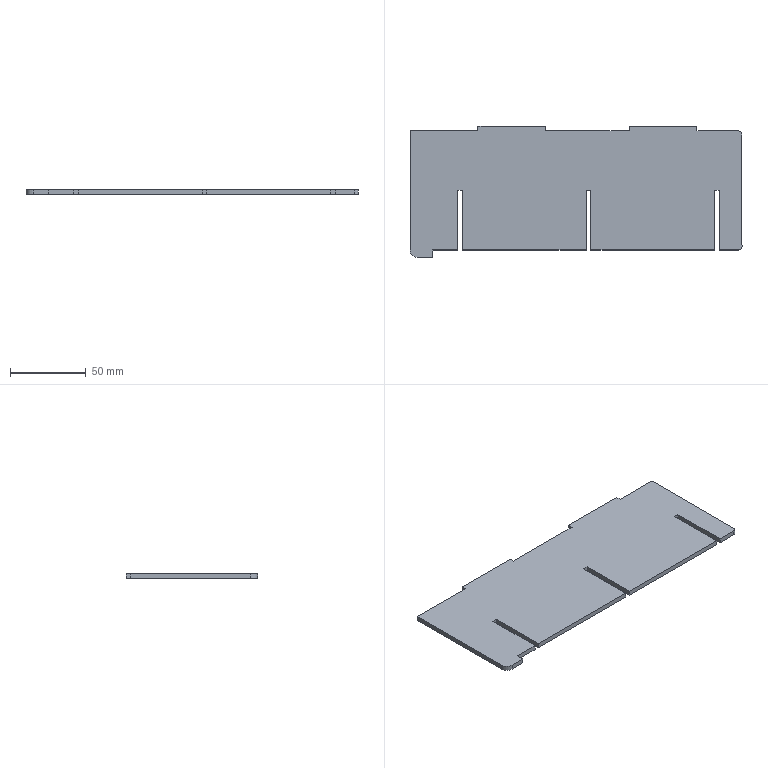Part | SolidWorks | features FlatPattern 1, SMBaseFlange 1, SheetMetal 1 | 1 solid | 31 faces | box 219.8 x 86.8 x 3.2 mm | volume 55293 mm3 | plane 28 | cylinder 3 | commonest cylinder face diameters 4 x2 10 x1
STEP:
#1=CARTESIAN_POINT('',(-115.113,-280.,0.));
#2=VERTEX_POINT('',#1);
#3=CARTESIAN_POINT('',(-98.513,-280.,0.));
#4=VERTEX_POINT('',#3);
#5=CARTESIAN_POINT('',(-98.513,-280.,0.));
#6=DIRECTION('',(1.,0.,0.));
#7=VECTOR('',#6,1000.);
#8=LINE('',#5,#7);
#9=EDGE_CURVE('',#2,#4,#8,.T.);
#10=ORIENTED_EDGE('',*,*,#9,.T.);
#11=CARTESIAN_POINT('',(-98.513,-280.,3.2));
#12=VERTEX_POINT('',#11);
#13=CARTESIAN_POINT('',(-98.513,-280.,3.2));
#14=DIRECTION('',(0.,0.,-1.));
#15=VECTOR('',#14,1000.);
#16=LINE('',#13,#15);
#17=EDGE_CURVE('',#12,#4,#16,.T.);
#18=ORIENTED_EDGE('',*,*,#17,.F.);
#19=CARTESIAN_POINT('',(-115.113,-280.,3.2));
#20=VERTEX_POINT('',#19);
#21=CARTESIAN_POINT('',(-98.513,-280.,3.2));
#22=DIRECTION('',(1.,0.,0.));
#23=VECTOR('',#22,1000.);
#24=LINE('',#21,#23);
#25=EDGE_CURVE('',#20,#12,#24,.T.);
#26=ORIENTED_EDGE('',*,*,#25,.F.);
#27=CARTESIAN_POINT('',(-115.113,-280.,3.2));
#28=DIRECTION('',(0.,0.,-1.));
#29=VECTOR('',#28,1000.);
#30=LINE('',#27,#29);
#31=EDGE_CURVE('',#20,#2,#30,.T.);
#32=ORIENTED_EDGE('',*,*,#31,.T.);
#33=EDGE_LOOP('',(#10,#18,#26,#32));
#34=FACE_OUTER_BOUND('',#33,.T.);
#35=CARTESIAN_POINT('',(-98.513,-280.,3.2));
#36=DIRECTION('',(0.,1.,0.));
#37=DIRECTION('',(-1.,0.,0.));
#38=AXIS2_PLACEMENT_3D('',#35,#36,#37);
#39=PLANE('',#38);
#40=ADVANCED_FACE('',(#34),#39,.F.);
#41=CARTESIAN_POINT('',(-98.513,-240.5,0.));
#42=VERTEX_POINT('',#41);
#43=CARTESIAN_POINT('',(-98.513,-280.,0.));
#44=DIRECTION('',(0.,1.,0.));
#45=VECTOR('',#44,1000.);
#46=LINE('',#43,#45);
#47=EDGE_CURVE('',#4,#42,#46,.T.);
#48=ORIENTED_EDGE('',*,*,#47,.T.);
#49=CARTESIAN_POINT('',(-98.513,-240.5,3.2));
#50=VERTEX_POINT('',#49);
#51=CARTESIAN_POINT('',(-98.513,-240.5,3.2));
#52=DIRECTION('',(0.,0.,-1.));
#53=VECTOR('',#52,1000.);
#54=LINE('',#51,#53);
#55=EDGE_CURVE('',#50,#42,#54,.T.);
#56=ORIENTED_EDGE('',*,*,#55,.F.);
#57=CARTESIAN_POINT('',(-98.513,-280.,3.2));
#58=DIRECTION('',(0.,1.,0.));
#59=VECTOR('',#58,1000.);
#60=LINE('',#57,#59);
#61=EDGE_CURVE('',#12,#50,#60,.T.);
#62=ORIENTED_EDGE('',*,*,#61,.F.);
#63=ORIENTED_EDGE('',*,*,#17,.T.);
#64=EDGE_LOOP('',(#48,#56,#62,#63));
#65=FACE_OUTER_BOUND('',#64,.T.);
#66=CARTESIAN_POINT('',(-98.513,-280.,3.2));
#67=DIRECTION('',(-1.,0.,0.));
#68=DIRECTION('',(0.,-1.,0.));
#69=AXIS2_PLACEMENT_3D('',#66,#67,#68);
#70=PLANE('',#69);
#71=ADVANCED_FACE('',(#65),#70,.F.);
#72=CARTESIAN_POINT('',(-95.313,-240.5,0.));
#73=VERTEX_POINT('',#72);
#74=CARTESIAN_POINT('',(-98.513,-240.5,0.));
#75=DIRECTION('',(1.,0.,0.));
#76=VECTOR('',#75,1000.);
#77=LINE('',#74,#76);
#78=EDGE_CURVE('',#42,#73,#77,.T.);
#79=ORIENTED_EDGE('',*,*,#78,.T.);
#80=CARTESIAN_POINT('',(-95.313,-240.5,3.2));
#81=VERTEX_POINT('',#80);
#82=CARTESIAN_POINT('',(-95.313,-240.5,3.2));
#83=DIRECTION('',(0.,0.,-1.));
#84=VECTOR('',#83,1000.);
#85=LINE('',#82,#84);
#86=EDGE_CURVE('',#81,#73,#85,.T.);
#87=ORIENTED_EDGE('',*,*,#86,.F.);
#88=CARTESIAN_POINT('',(-98.513,-240.5,3.2));
#89=DIRECTION('',(1.,0.,0.));
#90=VECTOR('',#89,1000.);
#91=LINE('',#88,#90);
#92=EDGE_CURVE('',#50,#81,#91,.T.);
#93=ORIENTED_EDGE('',*,*,#92,.F.);
#94=ORIENTED_EDGE('',*,*,#55,.T.);
#95=EDGE_LOOP('',(#79,#87,#93,#94));
#96=FACE_OUTER_BOUND('',#95,.T.);
#97=CARTESIAN_POINT('',(-98.513,-240.5,3.2));
#98=DIRECTION('',(0.,1.,0.));
#99=DIRECTION('',(0.,0.,1.));
#100=AXIS2_PLACEMENT_3D('',#97,#98,#99);
#101=PLANE('',#100);
#102=ADVANCED_FACE('',(#96),#101,.F.);
#103=CARTESIAN_POINT('',(-95.313,-280.,0.));
#104=VERTEX_POINT('',#103);
#105=CARTESIAN_POINT('',(-95.313,-240.5,0.));
#106=DIRECTION('',(0.,-1.,0.));
#107=VECTOR('',#106,1000.);
#108=LINE('',#105,#107);
#109=EDGE_CURVE('',#73,#104,#108,.T.);
#110=ORIENTED_EDGE('',*,*,#109,.T.);
#111=CARTESIAN_POINT('',(-95.313,-280.,3.2));
#112=VERTEX_POINT('',#111);
#113=CARTESIAN_POINT('',(-95.313,-280.,3.2));
#114=DIRECTION('',(0.,0.,-1.));
#115=VECTOR('',#114,1000.);
#116=LINE('',#113,#115);
#117=EDGE_CURVE('',#112,#104,#116,.T.);
#118=ORIENTED_EDGE('',*,*,#117,.F.);
#119=CARTESIAN_POINT('',(-95.313,-240.5,3.2));
#120=DIRECTION('',(0.,-1.,0.));
#121=VECTOR('',#120,1000.);
#122=LINE('',#119,#121);
#123=EDGE_CURVE('',#81,#112,#122,.T.);
#124=ORIENTED_EDGE('',*,*,#123,.F.);
#125=ORIENTED_EDGE('',*,*,#86,.T.);
#126=EDGE_LOOP('',(#110,#118,#124,#125));
#127=FACE_OUTER_BOUND('',#126,.T.);
#128=CARTESIAN_POINT('',(-95.313,-240.5,3.2));
#129=DIRECTION('',(1.,0.,0.));
#130=DIRECTION('',(0.,1.,0.));
#131=AXIS2_PLACEMENT_3D('',#128,#129,#130);
#132=PLANE('',#131);
#133=ADVANCED_FACE('',(#127),#132,.F.);
#134=CARTESIAN_POINT('',(-13.513,-280.,0.));
#135=VERTEX_POINT('',#134);
#136=CARTESIAN_POINT('',(-13.513,-280.,0.));
#137=DIRECTION('',(1.,0.,0.));
#138=VECTOR('',#137,1000.);
#139=LINE('',#136,#138);
#140=EDGE_CURVE('',#104,#135,#139,.T.);
#141=ORIENTED_EDGE('',*,*,#140,.T.);
#142=CARTESIAN_POINT('',(-13.513,-280.,3.2));
#143=VERTEX_POINT('',#142);
#144=CARTESIAN_POINT('',(-13.513,-280.,3.2));
#145=DIRECTION('',(0.,0.,-1.));
#146=VECTOR('',#145,1000.);
#147=LINE('',#144,#146);
#148=EDGE_CURVE('',#143,#135,#147,.T.);
#149=ORIENTED_EDGE('',*,*,#148,.F.);
#150=CARTESIAN_POINT('',(-13.513,-280.,3.2));
#151=DIRECTION('',(1.,0.,0.));
#152=VECTOR('',#151,1000.);
#153=LINE('',#150,#152);
#154=EDGE_CURVE('',#112,#143,#153,.T.);
#155=ORIENTED_EDGE('',*,*,#154,.F.);
#156=ORIENTED_EDGE('',*,*,#117,.T.);
#157=EDGE_LOOP('',(#141,#149,#155,#156));
#158=FACE_OUTER_BOUND('',#157,.T.);
#159=CARTESIAN_POINT('',(-13.513,-280.,3.2));
#160=DIRECTION('',(0.,1.,0.));
#161=DIRECTION('',(-1.,0.,0.));
#162=AXIS2_PLACEMENT_3D('',#159,#160,#161);
#163=PLANE('',#162);
#164=ADVANCED_FACE('',(#158),#163,.F.);
#165=CARTESIAN_POINT('',(-13.513,-240.5,0.));
#166=VERTEX_POINT('',#165);
#167=CARTESIAN_POINT('',(-13.513,-240.5,0.));
#168=DIRECTION('',(0.,1.,0.));
#169=VECTOR('',#168,1000.);
#170=LINE('',#167,#169);
#171=EDGE_CURVE('',#135,#166,#170,.T.);
#172=ORIENTED_EDGE('',*,*,#171,.T.);
#173=CARTESIAN_POINT('',(-13.513,-240.5,3.2));
#174=VERTEX_POINT('',#173);
#175=CARTESIAN_POINT('',(-13.513,-240.5,3.2));
#176=DIRECTION('',(0.,0.,-1.));
#177=VECTOR('',#176,1000.);
#178=LINE('',#175,#177);
#179=EDGE_CURVE('',#174,#166,#178,.T.);
#180=ORIENTED_EDGE('',*,*,#179,.F.);
#181=CARTESIAN_POINT('',(-13.513,-240.5,3.2));
#182=DIRECTION('',(0.,1.,0.));
#183=VECTOR('',#182,1000.);
#184=LINE('',#181,#183);
#185=EDGE_CURVE('',#143,#174,#184,.T.);
#186=ORIENTED_EDGE('',*,*,#185,.F.);
#187=ORIENTED_EDGE('',*,*,#148,.T.);
#188=EDGE_LOOP('',(#172,#180,#186,#187));
#189=FACE_OUTER_BOUND('',#188,.T.);
#190=CARTESIAN_POINT('',(-13.513,-240.5,3.2));
#191=DIRECTION('',(-1.,0.,0.));
#192=DIRECTION('',(0.,-1.,0.));
#193=AXIS2_PLACEMENT_3D('',#190,#191,#192);
#194=PLANE('',#193);
#195=ADVANCED_FACE('',(#189),#194,.F.);
#196=CARTESIAN_POINT('',(-10.313,-240.5,0.));
#197=VERTEX_POINT('',#196);
#198=CARTESIAN_POINT('',(-10.313,-240.5,0.));
#199=DIRECTION('',(1.,0.,0.));
#200=VECTOR('',#199,1000.);
#201=LINE('',#198,#200);
#202=EDGE_CURVE('',#166,#197,#201,.T.);
#203=ORIENTED_EDGE('',*,*,#202,.T.);
#204=CARTESIAN_POINT('',(-10.313,-240.5,3.2));
#205=VERTEX_POINT('',#204);
#206=CARTESIAN_POINT('',(-10.313,-240.5,3.2));
#207=DIRECTION('',(0.,0.,-1.));
#208=VECTOR('',#207,1000.);
#209=LINE('',#206,#208);
#210=EDGE_CURVE('',#205,#197,#209,.T.);
#211=ORIENTED_EDGE('',*,*,#210,.F.);
#212=CARTESIAN_POINT('',(-10.313,-240.5,3.2));
#213=DIRECTION('',(1.,0.,0.));
#214=VECTOR('',#213,1000.);
#215=LINE('',#212,#214);
#216=EDGE_CURVE('',#174,#205,#215,.T.);
#217=ORIENTED_EDGE('',*,*,#216,.F.);
#218=ORIENTED_EDGE('',*,*,#179,.T.);
#219=EDGE_LOOP('',(#203,#211,#217,#218));
#220=FACE_OUTER_BOUND('',#219,.T.);
#221=CARTESIAN_POINT('',(-10.313,-240.5,3.2));
#222=DIRECTION('',(0.,1.,0.));
#223=DIRECTION('',(0.,0.,1.));
#224=AXIS2_PLACEMENT_3D('',#221,#222,#223);
#225=PLANE('',#224);
#226=ADVANCED_FACE('',(#220),#225,.F.);
#227=CARTESIAN_POINT('',(-10.313,-280.,0.));
#228=VERTEX_POINT('',#227);
#229=CARTESIAN_POINT('',(-10.313,-280.,0.));
#230=DIRECTION('',(0.,-1.,0.));
#231=VECTOR('',#230,1000.);
#232=LINE('',#229,#231);
#233=EDGE_CURVE('',#197,#228,#232,.T.);
#234=ORIENTED_EDGE('',*,*,#233,.T.);
#235=CARTESIAN_POINT('',(-10.313,-280.,3.2));
#236=VERTEX_POINT('',#235);
#237=CARTESIAN_POINT('',(-10.313,-280.,3.2));
#238=DIRECTION('',(0.,0.,-1.));
#239=VECTOR('',#238,1000.);
#240=LINE('',#237,#239);
#241=EDGE_CURVE('',#236,#228,#240,.T.);
#242=ORIENTED_EDGE('',*,*,#241,.F.);
#243=CARTESIAN_POINT('',(-10.313,-280.,3.2));
#244=DIRECTION('',(0.,-1.,0.));
#245=VECTOR('',#244,1000.);
#246=LINE('',#243,#245);
#247=EDGE_CURVE('',#205,#236,#246,.T.);
#248=ORIENTED_EDGE('',*,*,#247,.F.);
#249=ORIENTED_EDGE('',*,*,#210,.T.);
#250=EDGE_LOOP('',(#234,#242,#248,#249));
#251=FACE_OUTER_BOUND('',#250,.T.);
#252=CARTESIAN_POINT('',(-10.313,-280.,3.2));
#253=DIRECTION('',(1.,0.,0.));
#254=DIRECTION('',(0.,1.,0.));
#255=AXIS2_PLACEMENT_3D('',#252,#253,#254);
#256=PLANE('',#255);
#257=ADVANCED_FACE('',(#251),#256,.F.);
#258=CARTESIAN_POINT('',(71.487,-280.,0.));
#259=VERTEX_POINT('',#258);
#260=CARTESIAN_POINT('',(71.487,-280.,0.));
#261=DIRECTION('',(1.,0.,0.));
#262=VECTOR('',#261,1000.);
#263=LINE('',#260,#262);
#264=EDGE_CURVE('',#228,#259,#263,.T.);
#265=ORIENTED_EDGE('',*,*,#264,.T.);
#266=CARTESIAN_POINT('',(71.487,-280.,3.2));
#267=VERTEX_POINT('',#266);
#268=CARTESIAN_POINT('',(71.487,-280.,3.2));
#269=DIRECTION('',(0.,0.,-1.));
#270=VECTOR('',#269,1000.);
#271=LINE('',#268,#270);
#272=EDGE_CURVE('',#267,#259,#271,.T.);
#273=ORIENTED_EDGE('',*,*,#272,.F.);
#274=CARTESIAN_POINT('',(71.487,-280.,3.2));
#275=DIRECTION('',(1.,0.,0.));
#276=VECTOR('',#275,1000.);
#277=LINE('',#274,#276);
#278=EDGE_CURVE('',#236,#267,#277,.T.);
#279=ORIENTED_EDGE('',*,*,#278,.F.);
#280=ORIENTED_EDGE('',*,*,#241,.T.);
#281=EDGE_LOOP('',(#265,#273,#279,#280));
#282=FACE_OUTER_BOUND('',#281,.T.);
#283=CARTESIAN_POINT('',(71.487,-280.,3.2));
#284=DIRECTION('',(0.,1.,0.));
#285=DIRECTION('',(-1.,0.,0.));
#286=AXIS2_PLACEMENT_3D('',#283,#284,#285);
#287=PLANE('',#286);
#288=ADVANCED_FACE('',(#282),#287,.F.);
#289=CARTESIAN_POINT('',(71.487,-240.5,0.));
#290=VERTEX_POINT('',#289);
#291=CARTESIAN_POINT('',(71.487,-280.,0.));
#292=DIRECTION('',(0.,1.,0.));
#293=VECTOR('',#292,1000.);
#294=LINE('',#291,#293);
#295=EDGE_CURVE('',#259,#290,#294,.T.);
#296=ORIENTED_EDGE('',*,*,#295,.T.);
#297=CARTESIAN_POINT('',(71.487,-240.5,3.2));
#298=VERTEX_POINT('',#297);
#299=CARTESIAN_POINT('',(71.487,-240.5,3.2));
#300=DIRECTION('',(0.,0.,-1.));
#301=VECTOR('',#300,1000.);
#302=LINE('',#299,#301);
#303=EDGE_CURVE('',#298,#290,#302,.T.);
#304=ORIENTED_EDGE('',*,*,#303,.F.);
#305=CARTESIAN_POINT('',(71.487,-280.,3.2));
#306=DIRECTION('',(0.,1.,0.));
#307=VECTOR('',#306,1000.);
#308=LINE('',#305,#307);
#309=EDGE_CURVE('',#267,#298,#308,.T.);
#310=ORIENTED_EDGE('',*,*,#309,.F.);
#311=ORIENTED_EDGE('',*,*,#272,.T.);
#312=EDGE_LOOP('',(#296,#304,#310,#311));
#313=FACE_OUTER_BOUND('',#312,.T.);
#314=CARTESIAN_POINT('',(71.487,-280.,3.2));
#315=DIRECTION('',(-1.,0.,0.));
#316=DIRECTION('',(0.,-1.,0.));
#317=AXIS2_PLACEMENT_3D('',#314,#315,#316);
#318=PLANE('',#317);
#319=ADVANCED_FACE('',(#313),#318,.F.);
#320=CARTESIAN_POINT('',(74.687,-240.5,0.));
#321=VERTEX_POINT('',#320);
#322=CARTESIAN_POINT('',(71.487,-240.5,0.));
#323=DIRECTION('',(1.,0.,0.));
#324=VECTOR('',#323,1000.);
#325=LINE('',#322,#324);
#326=EDGE_CURVE('',#290,#321,#325,.T.);
#327=ORIENTED_EDGE('',*,*,#326,.T.);
#328=CARTESIAN_POINT('',(74.687,-240.5,3.2));
#329=VERTEX_POINT('',#328);
#330=CARTESIAN_POINT('',(74.687,-240.5,3.2));
#331=DIRECTION('',(0.,0.,-1.));
#332=VECTOR('',#331,1000.);
#333=LINE('',#330,#332);
#334=EDGE_CURVE('',#329,#321,#333,.T.);
#335=ORIENTED_EDGE('',*,*,#334,.F.);
#336=CARTESIAN_POINT('',(71.487,-240.5,3.2));
#337=DIRECTION('',(1.,0.,0.));
#338=VECTOR('',#337,1000.);
#339=LINE('',#336,#338);
#340=EDGE_CURVE('',#298,#329,#339,.T.);
#341=ORIENTED_EDGE('',*,*,#340,.F.);
#342=ORIENTED_EDGE('',*,*,#303,.T.);
#343=EDGE_LOOP('',(#327,#335,#341,#342));
#344=FACE_OUTER_BOUND('',#343,.T.);
#345=CARTESIAN_POINT('',(71.487,-240.5,3.2));
#346=DIRECTION('',(0.,1.,0.));
#347=DIRECTION('',(0.,0.,1.));
#348=AXIS2_PLACEMENT_3D('',#345,#346,#347);
#349=PLANE('',#348);
#350=ADVANCED_FACE('',(#344),#349,.F.);
#351=CARTESIAN_POINT('',(74.687,-280.,0.));
#352=VERTEX_POINT('',#351);
#353=CARTESIAN_POINT('',(74.687,-240.5,0.));
#354=DIRECTION('',(0.,-1.,0.));
#355=VECTOR('',#354,1000.);
#356=LINE('',#353,#355);
#357=EDGE_CURVE('',#321,#352,#356,.T.);
#358=ORIENTED_EDGE('',*,*,#357,.T.);
#359=CARTESIAN_POINT('',(74.687,-280.,3.2));
#360=VERTEX_POINT('',#359);
#361=CARTESIAN_POINT('',(74.687,-280.,3.2));
#362=DIRECTION('',(0.,0.,-1.));
#363=VECTOR('',#362,1000.);
#364=LINE('',#361,#363);
#365=EDGE_CURVE('',#360,#352,#364,.T.);
#366=ORIENTED_EDGE('',*,*,#365,.F.);
#367=CARTESIAN_POINT('',(74.687,-240.5,3.2));
#368=DIRECTION('',(0.,-1.,0.));
#369=VECTOR('',#368,1000.);
#370=LINE('',#367,#369);
#371=EDGE_CURVE('',#329,#360,#370,.T.);
#372=ORIENTED_EDGE('',*,*,#371,.F.);
#373=ORIENTED_EDGE('',*,*,#334,.T.);
#374=EDGE_LOOP('',(#358,#366,#372,#373));
#375=FACE_OUTER_BOUND('',#374,.T.);
#376=CARTESIAN_POINT('',(74.687,-240.5,3.2));
#377=DIRECTION('',(1.,0.,0.));
#378=DIRECTION('',(0.,0.,-1.));
#379=AXIS2_PLACEMENT_3D('',#376,#377,#378);
#380=PLANE('',#379);
#381=ADVANCED_FACE('',(#375),#380,.F.);
#382=CARTESIAN_POINT('',(87.687,-280.,0.));
#383=VERTEX_POINT('',#382);
#384=CARTESIAN_POINT('',(87.687,-280.,0.));
#385=DIRECTION('',(1.,0.,0.));
#386=VECTOR('',#385,1000.);
#387=LINE('',#384,#386);
#388=EDGE_CURVE('',#352,#383,#387,.T.);
#389=ORIENTED_EDGE('',*,*,#388,.T.);
#390=CARTESIAN_POINT('',(87.687,-280.,3.2));
#391=VERTEX_POINT('',#390);
#392=CARTESIAN_POINT('',(87.687,-280.,3.2));
#393=DIRECTION('',(0.,0.,-1.));
#394=VECTOR('',#393,1000.);
#395=LINE('',#392,#394);
#396=EDGE_CURVE('',#391,#383,#395,.T.);
#397=ORIENTED_EDGE('',*,*,#396,.F.);
#398=CARTESIAN_POINT('',(87.687,-280.,3.2));
#399=DIRECTION('',(1.,0.,0.));
#400=VECTOR('',#399,1000.);
#401=LINE('',#398,#400);
#402=EDGE_CURVE('',#360,#391,#401,.T.);
#403=ORIENTED_EDGE('',*,*,#402,.F.);
#404=ORIENTED_EDGE('',*,*,#365,.T.);
#405=EDGE_LOOP('',(#389,#397,#403,#404));
#406=FACE_OUTER_BOUND('',#405,.T.);
#407=CARTESIAN_POINT('',(87.687,-280.,3.2));
#408=DIRECTION('',(0.,1.,0.));
#409=DIRECTION('',(-1.,0.,0.));
#410=AXIS2_PLACEMENT_3D('',#407,#408,#409);
#411=PLANE('',#410);
#412=ADVANCED_FACE('',(#406),#411,.F.);
#413=CARTESIAN_POINT('',(89.687,-278.,0.));
#414=VERTEX_POINT('',#413);
#415=CARTESIAN_POINT('',(87.687,-278.,0.));
#416=DIRECTION('',(0.,0.,1.));
#417=DIRECTION('',(1.,0.,0.));
#418=AXIS2_PLACEMENT_3D('',#415,#416,#417);
#419=CIRCLE('',#418,2.);
#420=EDGE_CURVE('',#383,#414,#419,.T.);
#421=ORIENTED_EDGE('',*,*,#420,.T.);
#422=CARTESIAN_POINT('',(89.687,-278.,3.2));
#423=VERTEX_POINT('',#422);
#424=CARTESIAN_POINT('',(89.687,-278.,3.2));
#425=DIRECTION('',(0.,0.,-1.));
#426=VECTOR('',#425,1000.);
#427=LINE('',#424,#426);
#428=EDGE_CURVE('',#423,#414,#427,.T.);
#429=ORIENTED_EDGE('',*,*,#428,.F.);
#430=CARTESIAN_POINT('',(87.687,-278.,3.2));
#431=DIRECTION('',(0.,0.,1.));
#432=DIRECTION('',(1.,0.,0.));
#433=AXIS2_PLACEMENT_3D('',#430,#431,#432);
#434=CIRCLE('',#433,2.);
#435=EDGE_CURVE('',#391,#423,#434,.T.);
#436=ORIENTED_EDGE('',*,*,#435,.F.);
#437=ORIENTED_EDGE('',*,*,#396,.T.);
#438=EDGE_LOOP('',(#421,#429,#436,#437));
#439=FACE_OUTER_BOUND('',#438,.T.);
#440=CARTESIAN_POINT('',(87.687,-278.,3.2));
#441=DIRECTION('',(0.,0.,-1.));
#442=DIRECTION('',(-1.,0.,0.));
#443=AXIS2_PLACEMENT_3D('',#440,#441,#442);
#444=CYLINDRICAL_SURFACE('',#443,2.);
#445=ADVANCED_FACE('',(#439),#444,.T.);
#446=CARTESIAN_POINT('',(89.687,-203.2,0.));
#447=VERTEX_POINT('',#446);
#448=CARTESIAN_POINT('',(89.687,-203.2,0.));
#449=DIRECTION('',(0.,1.,0.));
#450=VECTOR('',#449,1000.);
#451=LINE('',#448,#450);
#452=EDGE_CURVE('',#414,#447,#451,.T.);
#453=ORIENTED_EDGE('',*,*,#452,.T.);
#454=CARTESIAN_POINT('',(89.687,-203.2,3.2));
#455=VERTEX_POINT('',#454);
#456=CARTESIAN_POINT('',(89.687,-203.2,3.2));
#457=DIRECTION('',(0.,0.,-1.));
#458=VECTOR('',#457,1000.);
#459=LINE('',#456,#458);
#460=EDGE_CURVE('',#455,#447,#459,.T.);
#461=ORIENTED_EDGE('',*,*,#460,.F.);
#462=CARTESIAN_POINT('',(89.687,-203.2,3.2));
#463=DIRECTION('',(0.,1.,0.));
#464=VECTOR('',#463,1000.);
#465=LINE('',#462,#464);
#466=EDGE_CURVE('',#423,#455,#465,.T.);
#467=ORIENTED_EDGE('',*,*,#466,.F.);
#468=ORIENTED_EDGE('',*,*,#428,.T.);
#469=EDGE_LOOP('',(#453,#461,#467,#468));
#470=FACE_OUTER_BOUND('',#469,.T.);
#471=CARTESIAN_POINT('',(89.687,-203.2,3.2));
#472=DIRECTION('',(-1.,0.,0.));
#473=DIRECTION('',(0.,-1.,0.));
#474=AXIS2_PLACEMENT_3D('',#471,#472,#473);
#475=PLANE('',#474);
#476=ADVANCED_FACE('',(#470),#475,.F.);
#477=CARTESIAN_POINT('',(87.687,-201.2,0.));
#478=VERTEX_POINT('',#477);
#479=CARTESIAN_POINT('',(87.687,-203.2,0.));
#480=DIRECTION('',(0.,0.,1.));
#481=DIRECTION('',(-1.,0.,0.));
#482=AXIS2_PLACEMENT_3D('',#479,#480,#481);
#483=CIRCLE('',#482,2.);
#484=EDGE_CURVE('',#447,#478,#483,.T.);
#485=ORIENTED_EDGE('',*,*,#484,.T.);
#486=CARTESIAN_POINT('',(87.687,-201.2,3.2));
#487=VERTEX_POINT('',#486);
#488=CARTESIAN_POINT('',(87.687,-201.2,3.2));
#489=DIRECTION('',(0.,0.,-1.));
#490=VECTOR('',#489,1000.);
#491=LINE('',#488,#490);
#492=EDGE_CURVE('',#487,#478,#491,.T.);
#493=ORIENTED_EDGE('',*,*,#492,.F.);
#494=CARTESIAN_POINT('',(87.687,-203.2,3.2));
#495=DIRECTION('',(0.,0.,1.));
#496=DIRECTION('',(-1.,0.,0.));
#497=AXIS2_PLACEMENT_3D('',#494,#495,#496);
#498=CIRCLE('',#497,2.);
#499=EDGE_CURVE('',#455,#487,#498,.T.);
#500=ORIENTED_EDGE('',*,*,#499,.F.);
#501=ORIENTED_EDGE('',*,*,#460,.T.);
#502=EDGE_LOOP('',(#485,#493,#500,#501));
#503=FACE_OUTER_BOUND('',#502,.T.);
#504=CARTESIAN_POINT('',(87.687,-203.2,3.2));
#505=DIRECTION('',(0.,0.,-1.));
#506=DIRECTION('',(-1.,0.,0.));
#507=AXIS2_PLACEMENT_3D('',#504,#505,#506);
#508=CYLINDRICAL_SURFACE('',#507,2.);
#509=ADVANCED_FACE('',(#503),#508,.T.);
#510=CARTESIAN_POINT('',(59.887,-201.2,0.));
#511=VERTEX_POINT('',#510);
#512=CARTESIAN_POINT('',(59.887,-201.2,0.));
#513=DIRECTION('',(-1.,0.,0.));
#514=VECTOR('',#513,1000.);
#515=LINE('',#512,#514);
#516=EDGE_CURVE('',#478,#511,#515,.T.);
#517=ORIENTED_EDGE('',*,*,#516,.T.);
#518=CARTESIAN_POINT('',(59.887,-201.2,3.2));
#519=VERTEX_POINT('',#518);
#520=CARTESIAN_POINT('',(59.887,-201.2,3.2));
#521=DIRECTION('',(0.,0.,-1.));
#522=VECTOR('',#521,1000.);
#523=LINE('',#520,#522);
#524=EDGE_CURVE('',#519,#511,#523,.T.);
#525=ORIENTED_EDGE('',*,*,#524,.F.);
#526=CARTESIAN_POINT('',(59.887,-201.2,3.2));
#527=DIRECTION('',(-1.,0.,0.));
#528=VECTOR('',#527,1000.);
#529=LINE('',#526,#528);
#530=EDGE_CURVE('',#487,#519,#529,.T.);
#531=ORIENTED_EDGE('',*,*,#530,.F.);
#532=ORIENTED_EDGE('',*,*,#492,.T.);
#533=EDGE_LOOP('',(#517,#525,#531,#532));
#534=FACE_OUTER_BOUND('',#533,.T.);
#535=CARTESIAN_POINT('',(59.887,-201.2,3.2));
#536=DIRECTION('',(0.,-1.,0.));
#537=DIRECTION('',(1.,0.,0.));
#538=AXIS2_PLACEMENT_3D('',#535,#536,#537);
#539=PLANE('',#538);
#540=ADVANCED_FACE('',(#534),#539,.F.);
#541=CARTESIAN_POINT('',(59.887,-198.2,0.));
#542=VERTEX_POINT('',#541);
#543=CARTESIAN_POINT('',(59.887,-201.2,0.));
#544=DIRECTION('',(0.,1.,0.));
#545=VECTOR('',#544,1000.);
#546=LINE('',#543,#545);
#547=EDGE_CURVE('',#511,#542,#546,.T.);
#548=ORIENTED_EDGE('',*,*,#547,.T.);
#549=CARTESIAN_POINT('',(59.887,-198.2,3.2));
#550=VERTEX_POINT('',#549);
#551=CARTESIAN_POINT('',(59.887,-198.2,3.2));
#552=DIRECTION('',(0.,0.,-1.));
#553=VECTOR('',#552,1000.);
#554=LINE('',#551,#553);
#555=EDGE_CURVE('',#550,#542,#554,.T.);
#556=ORIENTED_EDGE('',*,*,#555,.F.);
#557=CARTESIAN_POINT('',(59.887,-201.2,3.2));
#558=DIRECTION('',(0.,1.,0.));
#559=VECTOR('',#558,1000.);
#560=LINE('',#557,#559);
#561=EDGE_CURVE('',#519,#550,#560,.T.);
#562=ORIENTED_EDGE('',*,*,#561,.F.);
#563=ORIENTED_EDGE('',*,*,#524,.T.);
#564=EDGE_LOOP('',(#548,#556,#562,#563));
#565=FACE_OUTER_BOUND('',#564,.T.);
#566=CARTESIAN_POINT('',(59.887,-201.2,3.2));
#567=DIRECTION('',(-1.,0.,0.));
#568=DIRECTION('',(0.,-1.,0.));
#569=AXIS2_PLACEMENT_3D('',#566,#567,#568);
#570=PLANE('',#569);
#571=ADVANCED_FACE('',(#565),#570,.F.);
#572=CARTESIAN_POINT('',(14.887,-198.2,0.));
#573=VERTEX_POINT('',#572);
#574=CARTESIAN_POINT('',(59.887,-198.2,0.));
#575=DIRECTION('',(-1.,0.,0.));
#576=VECTOR('',#575,1000.);
#577=LINE('',#574,#576);
#578=EDGE_CURVE('',#542,#573,#577,.T.);
#579=ORIENTED_EDGE('',*,*,#578,.T.);
#580=CARTESIAN_POINT('',(14.887,-198.2,3.2));
#581=VERTEX_POINT('',#580);
#582=CARTESIAN_POINT('',(14.887,-198.2,3.2));
#583=DIRECTION('',(0.,0.,-1.));
#584=VECTOR('',#583,1000.);
#585=LINE('',#582,#584);
#586=EDGE_CURVE('',#581,#573,#585,.T.);
#587=ORIENTED_EDGE('',*,*,#586,.F.);
#588=CARTESIAN_POINT('',(59.887,-198.2,3.2));
#589=DIRECTION('',(-1.,0.,0.));
#590=VECTOR('',#589,1000.);
#591=LINE('',#588,#590);
#592=EDGE_CURVE('',#550,#581,#591,.T.);
#593=ORIENTED_EDGE('',*,*,#592,.F.);
#594=ORIENTED_EDGE('',*,*,#555,.T.);
#595=EDGE_LOOP('',(#579,#587,#593,#594));
#596=FACE_OUTER_BOUND('',#595,.T.);
#597=CARTESIAN_POINT('',(59.887,-198.2,3.2));
#598=DIRECTION('',(0.,-1.,0.));
#599=DIRECTION('',(1.,0.,0.));
#600=AXIS2_PLACEMENT_3D('',#597,#598,#599);
#601=PLANE('',#600);
#602=ADVANCED_FACE('',(#596),#601,.F.);
#603=CARTESIAN_POINT('',(14.887,-201.2,0.));
#604=VERTEX_POINT('',#603);
#605=CARTESIAN_POINT('',(14.887,-198.2,0.));
#606=DIRECTION('',(0.,-1.,0.));
#607=VECTOR('',#606,1000.);
#608=LINE('',#605,#607);
#609=EDGE_CURVE('',#573,#604,#608,.T.);
#610=ORIENTED_EDGE('',*,*,#609,.T.);
#611=CARTESIAN_POINT('',(14.887,-201.2,3.2));
#612=VERTEX_POINT('',#611);
#613=CARTESIAN_POINT('',(14.887,-201.2,3.2));
#614=DIRECTION('',(0.,0.,-1.));
#615=VECTOR('',#614,1000.);
#616=LINE('',#613,#615);
#617=EDGE_CURVE('',#612,#604,#616,.T.);
#618=ORIENTED_EDGE('',*,*,#617,.F.);
#619=CARTESIAN_POINT('',(14.887,-198.2,3.2));
#620=DIRECTION('',(0.,-1.,0.));
#621=VECTOR('',#620,1000.);
#622=LINE('',#619,#621);
#623=EDGE_CURVE('',#581,#612,#622,.T.);
#624=ORIENTED_EDGE('',*,*,#623,.F.);
#625=ORIENTED_EDGE('',*,*,#586,.T.);
#626=EDGE_LOOP('',(#610,#618,#624,#625));
#627=FACE_OUTER_BOUND('',#626,.T.);
#628=CARTESIAN_POINT('',(14.887,-198.2,3.2));
#629=DIRECTION('',(1.,0.,0.));
#630=DIRECTION('',(0.,0.,-1.));
#631=AXIS2_PLACEMENT_3D('',#628,#629,#630);
#632=PLANE('',#631);
#633=ADVANCED_FACE('',(#627),#632,.F.);
#634=CARTESIAN_POINT('',(-40.113,-201.2,0.));
#635=VERTEX_POINT('',#634);
#636=CARTESIAN_POINT('',(-40.113,-201.2,0.));
#637=DIRECTION('',(-1.,0.,0.));
#638=VECTOR('',#637,1000.);
#639=LINE('',#636,#638);
#640=EDGE_CURVE('',#604,#635,#639,.T.);
#641=ORIENTED_EDGE('',*,*,#640,.T.);
#642=CARTESIAN_POINT('',(-40.113,-201.2,3.2));
#643=VERTEX_POINT('',#642);
#644=CARTESIAN_POINT('',(-40.113,-201.2,3.2));
#645=DIRECTION('',(0.,0.,-1.));
#646=VECTOR('',#645,1000.);
#647=LINE('',#644,#646);
#648=EDGE_CURVE('',#643,#635,#647,.T.);
#649=ORIENTED_EDGE('',*,*,#648,.F.);
#650=CARTESIAN_POINT('',(-40.113,-201.2,3.2));
#651=DIRECTION('',(-1.,0.,0.));
#652=VECTOR('',#651,1000.);
#653=LINE('',#650,#652);
#654=EDGE_CURVE('',#612,#643,#653,.T.);
#655=ORIENTED_EDGE('',*,*,#654,.F.);
#656=ORIENTED_EDGE('',*,*,#617,.T.);
#657=EDGE_LOOP('',(#641,#649,#655,#656));
#658=FACE_OUTER_BOUND('',#657,.T.);
#659=CARTESIAN_POINT('',(-40.113,-201.2,3.2));
#660=DIRECTION('',(0.,-1.,0.));
#661=DIRECTION('',(0.,0.,-1.));
#662=AXIS2_PLACEMENT_3D('',#659,#660,#661);
#663=PLANE('',#662);
#664=ADVANCED_FACE('',(#658),#663,.F.);
#665=CARTESIAN_POINT('',(-40.113,-198.2,0.));
#666=VERTEX_POINT('',#665);
#667=CARTESIAN_POINT('',(-40.113,-201.2,0.));
#668=DIRECTION('',(0.,1.,0.));
#669=VECTOR('',#668,1000.);
#670=LINE('',#667,#669);
#671=EDGE_CURVE('',#635,#666,#670,.T.);
#672=ORIENTED_EDGE('',*,*,#671,.T.);
#673=CARTESIAN_POINT('',(-40.113,-198.2,3.2));
#674=VERTEX_POINT('',#673);
#675=CARTESIAN_POINT('',(-40.113,-198.2,3.2));
#676=DIRECTION('',(0.,0.,-1.));
#677=VECTOR('',#676,1000.);
#678=LINE('',#675,#677);
#679=EDGE_CURVE('',#674,#666,#678,.T.);
#680=ORIENTED_EDGE('',*,*,#679,.F.);
#681=CARTESIAN_POINT('',(-40.113,-201.2,3.2));
#682=DIRECTION('',(0.,1.,0.));
#683=VECTOR('',#682,1000.);
#684=LINE('',#681,#683);
#685=EDGE_CURVE('',#643,#674,#684,.T.);
#686=ORIENTED_EDGE('',*,*,#685,.F.);
#687=ORIENTED_EDGE('',*,*,#648,.T.);
#688=EDGE_LOOP('',(#672,#680,#686,#687));
#689=FACE_OUTER_BOUND('',#688,.T.);
#690=CARTESIAN_POINT('',(-40.113,-201.2,3.2));
#691=DIRECTION('',(-1.,0.,0.));
#692=DIRECTION('',(0.,-1.,0.));
#693=AXIS2_PLACEMENT_3D('',#690,#691,#692);
#694=PLANE('',#693);
#695=ADVANCED_FACE('',(#689),#694,.F.);
#696=CARTESIAN_POINT('',(-85.113,-198.2,0.));
#697=VERTEX_POINT('',#696);
#698=CARTESIAN_POINT('',(-40.113,-198.2,0.));
#699=DIRECTION('',(-1.,0.,0.));
#700=VECTOR('',#699,1000.);
#701=LINE('',#698,#700);
#702=EDGE_CURVE('',#666,#697,#701,.T.);
#703=ORIENTED_EDGE('',*,*,#702,.T.);
#704=CARTESIAN_POINT('',(-85.113,-198.2,3.2));
#705=VERTEX_POINT('',#704);
#706=CARTESIAN_POINT('',(-85.113,-198.2,3.2));
#707=DIRECTION('',(0.,0.,-1.));
#708=VECTOR('',#707,1000.);
#709=LINE('',#706,#708);
#710=EDGE_CURVE('',#705,#697,#709,.T.);
#711=ORIENTED_EDGE('',*,*,#710,.F.);
#712=CARTESIAN_POINT('',(-40.113,-198.2,3.2));
#713=DIRECTION('',(-1.,0.,0.));
#714=VECTOR('',#713,1000.);
#715=LINE('',#712,#714);
#716=EDGE_CURVE('',#674,#705,#715,.T.);
#717=ORIENTED_EDGE('',*,*,#716,.F.);
#718=ORIENTED_EDGE('',*,*,#679,.T.);
#719=EDGE_LOOP('',(#703,#711,#717,#718));
#720=FACE_OUTER_BOUND('',#719,.T.);
#721=CARTESIAN_POINT('',(-40.113,-198.2,3.2));
#722=DIRECTION('',(0.,-1.,0.));
#723=DIRECTION('',(1.,0.,0.));
#724=AXIS2_PLACEMENT_3D('',#721,#722,#723);
#725=PLANE('',#724);
#726=ADVANCED_FACE('',(#720),#725,.F.);
#727=CARTESIAN_POINT('',(-85.113,-201.2,0.));
#728=VERTEX_POINT('',#727);
#729=CARTESIAN_POINT('',(-85.113,-198.2,0.));
#730=DIRECTION('',(0.,-1.,0.));
#731=VECTOR('',#730,1000.);
#732=LINE('',#729,#731);
#733=EDGE_CURVE('',#697,#728,#732,.T.);
#734=ORIENTED_EDGE('',*,*,#733,.T.);
#735=CARTESIAN_POINT('',(-85.113,-201.2,3.2));
#736=VERTEX_POINT('',#735);
#737=CARTESIAN_POINT('',(-85.113,-201.2,3.2));
#738=DIRECTION('',(0.,0.,-1.));
#739=VECTOR('',#738,1000.);
#740=LINE('',#737,#739);
#741=EDGE_CURVE('',#736,#728,#740,.T.);
#742=ORIENTED_EDGE('',*,*,#741,.F.);
#743=CARTESIAN_POINT('',(-85.113,-198.2,3.2));
#744=DIRECTION('',(0.,-1.,0.));
#745=VECTOR('',#744,1000.);
#746=LINE('',#743,#745);
#747=EDGE_CURVE('',#705,#736,#746,.T.);
#748=ORIENTED_EDGE('',*,*,#747,.F.);
#749=ORIENTED_EDGE('',*,*,#710,.T.);
#750=EDGE_LOOP('',(#734,#742,#748,#749));
#751=FACE_OUTER_BOUND('',#750,.T.);
#752=CARTESIAN_POINT('',(-85.113,-198.2,3.2));
#753=DIRECTION('',(1.,0.,0.));
#754=DIRECTION('',(0.,0.,-1.));
#755=AXIS2_PLACEMENT_3D('',#752,#753,#754);
#756=PLANE('',#755);
#757=ADVANCED_FACE('',(#751),#756,.F.);
#758=CARTESIAN_POINT('',(-130.113,-201.2,0.));
#759=VERTEX_POINT('',#758);
#760=CARTESIAN_POINT('',(-130.113,-201.2,0.));
#761=DIRECTION('',(-1.,0.,0.));
#762=VECTOR('',#761,1000.);
#763=LINE('',#760,#762);
#764=EDGE_CURVE('',#728,#759,#763,.T.);
#765=ORIENTED_EDGE('',*,*,#764,.T.);
#766=CARTESIAN_POINT('',(-130.113,-201.2,3.2));
#767=VERTEX_POINT('',#766);
#768=CARTESIAN_POINT('',(-130.113,-201.2,3.2));
#769=DIRECTION('',(0.,0.,-1.));
#770=VECTOR('',#769,1000.);
#771=LINE('',#768,#770);
#772=EDGE_CURVE('',#767,#759,#771,.T.);
#773=ORIENTED_EDGE('',*,*,#772,.F.);
#774=CARTESIAN_POINT('',(-130.113,-201.2,3.2));
#775=DIRECTION('',(-1.,0.,0.));
#776=VECTOR('',#775,1000.);
#777=LINE('',#774,#776);
#778=EDGE_CURVE('',#736,#767,#777,.T.);
#779=ORIENTED_EDGE('',*,*,#778,.F.);
#780=ORIENTED_EDGE('',*,*,#741,.T.);
#781=EDGE_LOOP('',(#765,#773,#779,#780));
#782=FACE_OUTER_BOUND('',#781,.T.);
#783=CARTESIAN_POINT('',(-130.113,-201.2,3.2));
#784=DIRECTION('',(0.,-1.,0.));
#785=DIRECTION('',(0.,0.,-1.));
#786=AXIS2_PLACEMENT_3D('',#783,#784,#785);
#787=PLANE('',#786);
#788=ADVANCED_FACE('',(#782),#787,.F.);
#789=CARTESIAN_POINT('',(-130.113,-280.,0.));
#790=VERTEX_POINT('',#789);
#791=CARTESIAN_POINT('',(-130.113,-280.,0.));
#792=DIRECTION('',(0.,-1.,0.));
#793=VECTOR('',#792,1000.);
#794=LINE('',#791,#793);
#795=EDGE_CURVE('',#759,#790,#794,.T.);
#796=ORIENTED_EDGE('',*,*,#795,.T.);
#797=CARTESIAN_POINT('',(-130.113,-280.,3.2));
#798=VERTEX_POINT('',#797);
#799=CARTESIAN_POINT('',(-130.113,-280.,3.2));
#800=DIRECTION('',(0.,0.,-1.));
#801=VECTOR('',#800,1000.);
#802=LINE('',#799,#801);
#803=EDGE_CURVE('',#798,#790,#802,.T.);
#804=ORIENTED_EDGE('',*,*,#803,.F.);
#805=CARTESIAN_POINT('',(-130.113,-280.,3.2));
#806=DIRECTION('',(0.,-1.,0.));
#807=VECTOR('',#806,1000.);
#808=LINE('',#805,#807);
#809=EDGE_CURVE('',#767,#798,#808,.T.);
#810=ORIENTED_EDGE('',*,*,#809,.F.);
#811=ORIENTED_EDGE('',*,*,#772,.T.);
#812=EDGE_LOOP('',(#796,#804,#810,#811));
#813=FACE_OUTER_BOUND('',#812,.T.);
#814=CARTESIAN_POINT('',(-130.113,-280.,3.2));
#815=DIRECTION('',(1.,0.,0.));
#816=DIRECTION('',(0.,1.,0.));
#817=AXIS2_PLACEMENT_3D('',#814,#815,#816);
#818=PLANE('',#817);
#819=ADVANCED_FACE('',(#813),#818,.F.);
#820=CARTESIAN_POINT('',(-125.113,-285.,0.));
#821=VERTEX_POINT('',#820);
#822=CARTESIAN_POINT('',(-125.113,-280.,0.));
#823=DIRECTION('',(0.,0.,1.));
#824=DIRECTION('',(-1.,0.,0.));
#825=AXIS2_PLACEMENT_3D('',#822,#823,#824);
#826=CIRCLE('',#825,5.);
#827=EDGE_CURVE('',#790,#821,#826,.T.);
#828=ORIENTED_EDGE('',*,*,#827,.T.);
#829=CARTESIAN_POINT('',(-125.113,-285.,3.2));
#830=VERTEX_POINT('',#829);
#831=CARTESIAN_POINT('',(-125.113,-285.,3.2));
#832=DIRECTION('',(0.,0.,-1.));
#833=VECTOR('',#832,1000.);
#834=LINE('',#831,#833);
#835=EDGE_CURVE('',#830,#821,#834,.T.);
#836=ORIENTED_EDGE('',*,*,#835,.F.);
#837=CARTESIAN_POINT('',(-125.113,-280.,3.2));
#838=DIRECTION('',(0.,0.,1.));
#839=DIRECTION('',(-1.,0.,0.));
#840=AXIS2_PLACEMENT_3D('',#837,#838,#839);
#841=CIRCLE('',#840,5.);
#842=EDGE_CURVE('',#798,#830,#841,.T.);
#843=ORIENTED_EDGE('',*,*,#842,.F.);
#844=ORIENTED_EDGE('',*,*,#803,.T.);
#845=EDGE_LOOP('',(#828,#836,#843,#844));
#846=FACE_OUTER_BOUND('',#845,.T.);
#847=CARTESIAN_POINT('',(-125.113,-280.,3.2));
#848=DIRECTION('',(0.,0.,-1.));
#849=DIRECTION('',(-1.,0.,0.));
#850=AXIS2_PLACEMENT_3D('',#847,#848,#849);
#851=CYLINDRICAL_SURFACE('',#850,5.);
#852=ADVANCED_FACE('',(#846),#851,.T.);
#853=CARTESIAN_POINT('',(-115.113,-285.,0.));
#854=VERTEX_POINT('',#853);
#855=CARTESIAN_POINT('',(-115.113,-285.,0.));
#856=DIRECTION('',(1.,0.,0.));
#857=VECTOR('',#856,1000.);
#858=LINE('',#855,#857);
#859=EDGE_CURVE('',#821,#854,#858,.T.);
#860=ORIENTED_EDGE('',*,*,#859,.T.);
#861=CARTESIAN_POINT('',(-115.113,-285.,3.2));
#862=VERTEX_POINT('',#861);
#863=CARTESIAN_POINT('',(-115.113,-285.,3.2));
#864=DIRECTION('',(0.,0.,-1.));
#865=VECTOR('',#864,1000.);
#866=LINE('',#863,#865);
#867=EDGE_CURVE('',#862,#854,#866,.T.);
#868=ORIENTED_EDGE('',*,*,#867,.F.);
#869=CARTESIAN_POINT('',(-115.113,-285.,3.2));
#870=DIRECTION('',(1.,0.,0.));
#871=VECTOR('',#870,1000.);
#872=LINE('',#869,#871);
#873=EDGE_CURVE('',#830,#862,#872,.T.);
#874=ORIENTED_EDGE('',*,*,#873,.F.);
#875=ORIENTED_EDGE('',*,*,#835,.T.);
#876=EDGE_LOOP('',(#860,#868,#874,#875));
#877=FACE_OUTER_BOUND('',#876,.T.);
#878=CARTESIAN_POINT('',(-115.113,-285.,3.2));
#879=DIRECTION('',(0.,1.,0.));
#880=DIRECTION('',(0.,0.,1.));
#881=AXIS2_PLACEMENT_3D('',#878,#879,#880);
#882=PLANE('',#881);
#883=ADVANCED_FACE('',(#877),#882,.F.);
#884=CARTESIAN_POINT('',(-115.113,-280.,0.));
#885=DIRECTION('',(0.,1.,0.));
#886=VECTOR('',#885,1000.);
#887=LINE('',#884,#886);
#888=EDGE_CURVE('',#854,#2,#887,.T.);
#889=ORIENTED_EDGE('',*,*,#888,.T.);
#890=ORIENTED_EDGE('',*,*,#31,.F.);
#891=CARTESIAN_POINT('',(-115.113,-280.,3.2));
#892=DIRECTION('',(0.,1.,0.));
#893=VECTOR('',#892,1000.);
#894=LINE('',#891,#893);
#895=EDGE_CURVE('',#862,#20,#894,.T.);
#896=ORIENTED_EDGE('',*,*,#895,.F.);
#897=ORIENTED_EDGE('',*,*,#867,.T.);
#898=EDGE_LOOP('',(#889,#890,#896,#897));
#899=FACE_OUTER_BOUND('',#898,.T.);
#900=CARTESIAN_POINT('',(-115.113,-280.,3.2));
#901=DIRECTION('',(-1.,0.,0.));
#902=DIRECTION('',(0.,-1.,0.));
#903=AXIS2_PLACEMENT_3D('',#900,#901,#902);
#904=PLANE('',#903);
#905=ADVANCED_FACE('',(#899),#904,.F.);
#906=ORIENTED_EDGE('',*,*,#25,.T.);
#907=ORIENTED_EDGE('',*,*,#61,.T.);
#908=ORIENTED_EDGE('',*,*,#92,.T.);
#909=ORIENTED_EDGE('',*,*,#123,.T.);
#910=ORIENTED_EDGE('',*,*,#154,.T.);
#911=ORIENTED_EDGE('',*,*,#185,.T.);
#912=ORIENTED_EDGE('',*,*,#216,.T.);
#913=ORIENTED_EDGE('',*,*,#247,.T.);
#914=ORIENTED_EDGE('',*,*,#278,.T.);
#915=ORIENTED_EDGE('',*,*,#309,.T.);
#916=ORIENTED_EDGE('',*,*,#340,.T.);
#917=ORIENTED_EDGE('',*,*,#371,.T.);
#918=ORIENTED_EDGE('',*,*,#402,.T.);
#919=ORIENTED_EDGE('',*,*,#435,.T.);
#920=ORIENTED_EDGE('',*,*,#466,.T.);
#921=ORIENTED_EDGE('',*,*,#499,.T.);
#922=ORIENTED_EDGE('',*,*,#530,.T.);
#923=ORIENTED_EDGE('',*,*,#561,.T.);
#924=ORIENTED_EDGE('',*,*,#592,.T.);
#925=ORIENTED_EDGE('',*,*,#623,.T.);
#926=ORIENTED_EDGE('',*,*,#654,.T.);
#927=ORIENTED_EDGE('',*,*,#685,.T.);
#928=ORIENTED_EDGE('',*,*,#716,.T.);
#929=ORIENTED_EDGE('',*,*,#747,.T.);
#930=ORIENTED_EDGE('',*,*,#778,.T.);
#931=ORIENTED_EDGE('',*,*,#809,.T.);
#932=ORIENTED_EDGE('',*,*,#842,.T.);
#933=ORIENTED_EDGE('',*,*,#873,.T.);
#934=ORIENTED_EDGE('',*,*,#895,.T.);
#935=EDGE_LOOP('',(#906,#907,#908,#909,#910,#911,#912,#913,#914,#915,#916,#917,#918,#919,#920,#921,#922,#923,#924,#925,#926,#927,#928,#929,#930,#931,#932,#933,#934));
#936=FACE_OUTER_BOUND('',#935,.T.);
#937=CARTESIAN_POINT('',(-125.113,-280.,3.2));
#938=DIRECTION('',(0.,0.,-1.));
#939=DIRECTION('',(-1.,0.,0.));
#940=AXIS2_PLACEMENT_3D('',#937,#938,#939);
#941=PLANE('',#940);
#942=ADVANCED_FACE('',(#936),#941,.F.);
#943=ORIENTED_EDGE('',*,*,#9,.F.);
#944=ORIENTED_EDGE('',*,*,#888,.F.);
#945=ORIENTED_EDGE('',*,*,#859,.F.);
#946=ORIENTED_EDGE('',*,*,#827,.F.);
#947=ORIENTED_EDGE('',*,*,#795,.F.);
#948=ORIENTED_EDGE('',*,*,#764,.F.);
#949=ORIENTED_EDGE('',*,*,#733,.F.);
#950=ORIENTED_EDGE('',*,*,#702,.F.);
#951=ORIENTED_EDGE('',*,*,#671,.F.);
#952=ORIENTED_EDGE('',*,*,#640,.F.);
#953=ORIENTED_EDGE('',*,*,#609,.F.);
#954=ORIENTED_EDGE('',*,*,#578,.F.);
#955=ORIENTED_EDGE('',*,*,#547,.F.);
#956=ORIENTED_EDGE('',*,*,#516,.F.);
#957=ORIENTED_EDGE('',*,*,#484,.F.);
#958=ORIENTED_EDGE('',*,*,#452,.F.);
#959=ORIENTED_EDGE('',*,*,#420,.F.);
#960=ORIENTED_EDGE('',*,*,#388,.F.);
#961=ORIENTED_EDGE('',*,*,#357,.F.);
#962=ORIENTED_EDGE('',*,*,#326,.F.);
#963=ORIENTED_EDGE('',*,*,#295,.F.);
#964=ORIENTED_EDGE('',*,*,#264,.F.);
#965=ORIENTED_EDGE('',*,*,#233,.F.);
#966=ORIENTED_EDGE('',*,*,#202,.F.);
#967=ORIENTED_EDGE('',*,*,#171,.F.);
#968=ORIENTED_EDGE('',*,*,#140,.F.);
#969=ORIENTED_EDGE('',*,*,#109,.F.);
#970=ORIENTED_EDGE('',*,*,#78,.F.);
#971=ORIENTED_EDGE('',*,*,#47,.F.);
#972=EDGE_LOOP('',(#943,#944,#945,#946,#947,#948,#949,#950,#951,#952,#953,#954,#955,#956,#957,#958,#959,#960,#961,#962,#963,#964,#965,#966,#967,#968,#969,#970,#971));
#973=FACE_OUTER_BOUND('',#972,.T.);
#974=CARTESIAN_POINT('',(-125.113,-280.,0.));
#975=DIRECTION('',(0.,0.,-1.));
#976=DIRECTION('',(-1.,0.,0.));
#977=AXIS2_PLACEMENT_3D('',#974,#975,#976);
#978=PLANE('',#977);
#979=ADVANCED_FACE('',(#973),#978,.T.);
#980=CLOSED_SHELL('',(#40,#71,#102,#133,#164,#195,#226,#257,#288,#319,#350,#381,#412,#445,#476,#509,#540,#571,#602,#633,#664,#695,#726,#757,#788,#819,#852,#883,#905,#942,#979));
#981=MANIFOLD_SOLID_BREP('',#980);
#982=CARTESIAN_POINT('',(0.,0.,0.));
#983=DIRECTION('',(0.,0.,1.));
#984=DIRECTION('',(1.,0.,0.));
#985=AXIS2_PLACEMENT_3D('',#982,#983,#984);
#986=(LENGTH_UNIT()NAMED_UNIT(*)SI_UNIT(.MILLI.,.METRE.));
#987=UNCERTAINTY_MEASURE_WITH_UNIT(LENGTH_MEASURE(0.00001),#986,'','');
#988=(NAMED_UNIT(*)PLANE_ANGLE_UNIT()SI_UNIT($,.RADIAN.));
#989=(NAMED_UNIT(*)SI_UNIT($,.STERADIAN.)SOLID_ANGLE_UNIT());
#990=(GEOMETRIC_REPRESENTATION_CONTEXT(3)GLOBAL_UNCERTAINTY_ASSIGNED_CONTEXT((#987))GLOBAL_UNIT_ASSIGNED_CONTEXT((#986,#988,#989))REPRESENTATION_CONTEXT('',''));
#991=ADVANCED_BREP_SHAPE_REPRESENTATION('',(#981,#985),#990);